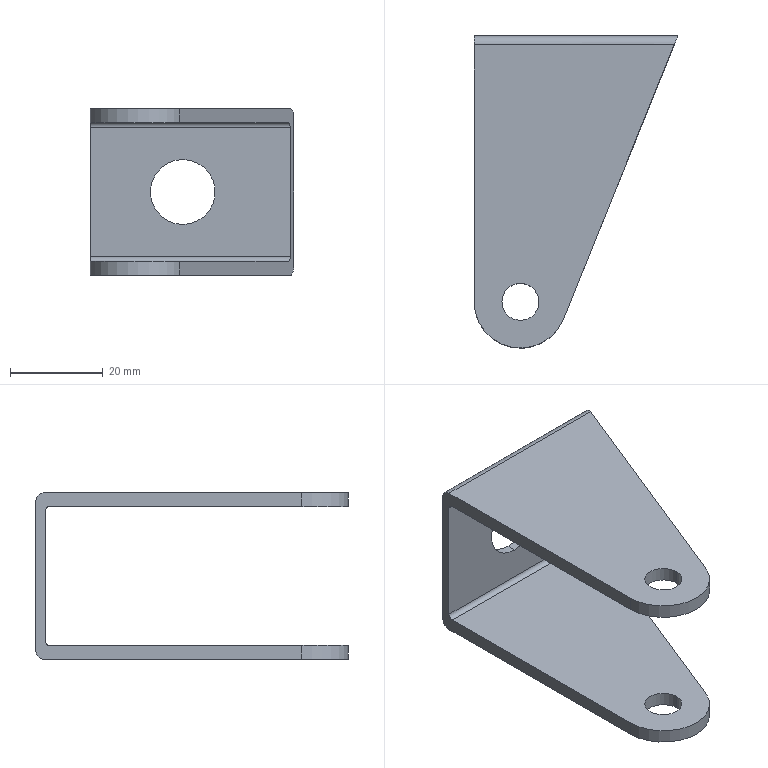Part | SolidWorks | features ICE 2, Extrusion 1, Fillet 1 | 1 solid | 20 faces | box 44 x 67.458 x 36 mm | volume 14065 mm3 | cylinder 12 | plane 8 | commonest cylinder face diameters 8 x4 2 x2 4 x2 14 x2 20 x2
STEP:
#1=CARTESIAN_POINT('',(20.,-2.,-25.));
#2=VERTEX_POINT('',#1);
#3=CARTESIAN_POINT('',(20.,-2.,-11.));
#4=VERTEX_POINT('',#3);
#5=CARTESIAN_POINT('',(20.,-2.,-18.));
#6=DIRECTION('',(0.,1.,0.));
#7=DIRECTION('',(-1.,0.,0.));
#8=AXIS2_PLACEMENT_3D('',#5,#6,#7);
#9=CIRCLE('',#8,7.);
#10=EDGE_CURVE('',#2,#4,#9,.T.);
#11=ORIENTED_EDGE('',*,*,#10,.F.);
#12=CARTESIAN_POINT('',(20.,0.,-25.));
#13=VERTEX_POINT('',#12);
#14=CARTESIAN_POINT('',(20.,-57.,-25.));
#15=DIRECTION('',(0.,1.,0.));
#16=VECTOR('',#15,1000.);
#17=LINE('',#14,#16);
#18=EDGE_CURVE('',#2,#13,#17,.T.);
#19=ORIENTED_EDGE('',*,*,#18,.T.);
#20=CARTESIAN_POINT('',(20.,0.,-11.));
#21=VERTEX_POINT('',#20);
#22=CARTESIAN_POINT('',(20.,0.,-18.));
#23=DIRECTION('',(0.,1.,0.));
#24=DIRECTION('',(0.,0.,1.));
#25=AXIS2_PLACEMENT_3D('',#22,#23,#24);
#26=CIRCLE('',#25,7.);
#27=EDGE_CURVE('',#13,#21,#26,.T.);
#28=ORIENTED_EDGE('',*,*,#27,.T.);
#29=CARTESIAN_POINT('',(20.,-57.,-11.));
#30=DIRECTION('',(0.,1.,0.));
#31=VECTOR('',#30,1000.);
#32=LINE('',#29,#31);
#33=EDGE_CURVE('',#4,#21,#32,.T.);
#34=ORIENTED_EDGE('',*,*,#33,.F.);
#35=EDGE_LOOP('',(#11,#19,#28,#34));
#36=FACE_OUTER_BOUND('',#35,.T.);
#37=CARTESIAN_POINT('',(20.,-57.,-18.));
#38=DIRECTION('',(0.,1.,0.));
#39=DIRECTION('',(0.,0.,1.));
#40=AXIS2_PLACEMENT_3D('',#37,#38,#39);
#41=CYLINDRICAL_SURFACE('',#40,7.);
#42=ADVANCED_FACE('',(#36),#41,.F.);
#43=CARTESIAN_POINT('',(14.,-57.458,-3.));
#44=VERTEX_POINT('',#43);
#45=CARTESIAN_POINT('',(6.,-57.458,-3.));
#46=VERTEX_POINT('',#45);
#47=CARTESIAN_POINT('',(10.,-57.458,-3.));
#48=DIRECTION('',(0.,0.,-1.));
#49=DIRECTION('',(0.,-1.,0.));
#50=AXIS2_PLACEMENT_3D('',#47,#48,#49);
#51=CIRCLE('',#50,4.);
#52=EDGE_CURVE('',#44,#46,#51,.T.);
#53=ORIENTED_EDGE('',*,*,#52,.T.);
#54=CARTESIAN_POINT('',(6.,-57.458,0.));
#55=VERTEX_POINT('',#54);
#56=CARTESIAN_POINT('',(6.,-57.458,-36.));
#57=DIRECTION('',(0.,0.,1.));
#58=VECTOR('',#57,1000.);
#59=LINE('',#56,#58);
#60=EDGE_CURVE('',#46,#55,#59,.T.);
#61=ORIENTED_EDGE('',*,*,#60,.T.);
#62=CARTESIAN_POINT('',(14.,-57.458,0.));
#63=VERTEX_POINT('',#62);
#64=CARTESIAN_POINT('',(10.,-57.458,0.));
#65=DIRECTION('',(0.,0.,1.));
#66=DIRECTION('',(1.,0.,0.));
#67=AXIS2_PLACEMENT_3D('',#64,#65,#66);
#68=CIRCLE('',#67,4.);
#69=EDGE_CURVE('',#55,#63,#68,.T.);
#70=ORIENTED_EDGE('',*,*,#69,.T.);
#71=CARTESIAN_POINT('',(14.,-57.458,-36.));
#72=DIRECTION('',(0.,0.,1.));
#73=VECTOR('',#72,1000.);
#74=LINE('',#71,#73);
#75=EDGE_CURVE('',#44,#63,#74,.T.);
#76=ORIENTED_EDGE('',*,*,#75,.F.);
#77=EDGE_LOOP('',(#53,#61,#70,#76));
#78=FACE_OUTER_BOUND('',#77,.T.);
#79=CARTESIAN_POINT('',(10.,-57.458,-36.));
#80=DIRECTION('',(0.,0.,1.));
#81=DIRECTION('',(1.,0.,0.));
#82=AXIS2_PLACEMENT_3D('',#79,#80,#81);
#83=CYLINDRICAL_SURFACE('',#82,4.);
#84=ADVANCED_FACE('',(#78),#83,.F.);
#85=CARTESIAN_POINT('',(6.,-57.458,-36.));
#86=VERTEX_POINT('',#85);
#87=CARTESIAN_POINT('',(14.,-57.458,-36.));
#88=VERTEX_POINT('',#87);
#89=CARTESIAN_POINT('',(10.,-57.458,-36.));
#90=DIRECTION('',(0.,0.,1.));
#91=DIRECTION('',(1.,0.,0.));
#92=AXIS2_PLACEMENT_3D('',#89,#90,#91);
#93=CIRCLE('',#92,4.);
#94=EDGE_CURVE('',#86,#88,#93,.T.);
#95=ORIENTED_EDGE('',*,*,#94,.F.);
#96=CARTESIAN_POINT('',(6.,-57.458,-33.));
#97=VERTEX_POINT('',#96);
#98=CARTESIAN_POINT('',(6.,-57.458,-36.));
#99=DIRECTION('',(0.,0.,1.));
#100=VECTOR('',#99,1000.);
#101=LINE('',#98,#100);
#102=EDGE_CURVE('',#86,#97,#101,.T.);
#103=ORIENTED_EDGE('',*,*,#102,.T.);
#104=CARTESIAN_POINT('',(14.,-57.458,-33.));
#105=VERTEX_POINT('',#104);
#106=CARTESIAN_POINT('',(10.,-57.458,-33.));
#107=DIRECTION('',(0.,0.,1.));
#108=DIRECTION('',(-1.,0.,0.));
#109=AXIS2_PLACEMENT_3D('',#106,#107,#108);
#110=CIRCLE('',#109,4.);
#111=EDGE_CURVE('',#97,#105,#110,.T.);
#112=ORIENTED_EDGE('',*,*,#111,.T.);
#113=CARTESIAN_POINT('',(14.,-57.458,-36.));
#114=DIRECTION('',(0.,0.,1.));
#115=VECTOR('',#114,1000.);
#116=LINE('',#113,#115);
#117=EDGE_CURVE('',#88,#105,#116,.T.);
#118=ORIENTED_EDGE('',*,*,#117,.F.);
#119=EDGE_LOOP('',(#95,#103,#112,#118));
#120=FACE_OUTER_BOUND('',#119,.T.);
#121=CARTESIAN_POINT('',(10.,-57.458,-36.));
#122=DIRECTION('',(0.,0.,1.));
#123=DIRECTION('',(1.,0.,0.));
#124=AXIS2_PLACEMENT_3D('',#121,#122,#123);
#125=CYLINDRICAL_SURFACE('',#124,4.);
#126=ADVANCED_FACE('',(#120),#125,.F.);
#127=CARTESIAN_POINT('',(0.,-57.458,-33.));
#128=VERTEX_POINT('',#127);
#129=CARTESIAN_POINT('',(19.272,-61.204,-33.));
#130=VERTEX_POINT('',#129);
#131=CARTESIAN_POINT('',(10.,-57.458,-33.));
#132=DIRECTION('',(0.,0.,1.));
#133=DIRECTION('',(-1.,0.,0.));
#134=AXIS2_PLACEMENT_3D('',#131,#132,#133);
#135=CIRCLE('',#134,10.);
#136=EDGE_CURVE('',#128,#130,#135,.T.);
#137=ORIENTED_EDGE('',*,*,#136,.F.);
#138=CARTESIAN_POINT('',(0.,-57.458,-36.));
#139=VERTEX_POINT('',#138);
#140=CARTESIAN_POINT('',(0.,-57.458,-36.));
#141=DIRECTION('',(0.,0.,1.));
#142=VECTOR('',#141,1000.);
#143=LINE('',#140,#142);
#144=EDGE_CURVE('',#139,#128,#143,.T.);
#145=ORIENTED_EDGE('',*,*,#144,.F.);
#146=CARTESIAN_POINT('',(19.272,-61.204,-36.));
#147=VERTEX_POINT('',#146);
#148=CARTESIAN_POINT('',(10.,-57.458,-36.));
#149=DIRECTION('',(0.,0.,1.));
#150=DIRECTION('',(1.,0.,0.));
#151=AXIS2_PLACEMENT_3D('',#148,#149,#150);
#152=CIRCLE('',#151,10.);
#153=EDGE_CURVE('',#139,#147,#152,.T.);
#154=ORIENTED_EDGE('',*,*,#153,.T.);
#155=CARTESIAN_POINT('',(19.272,-61.204,-36.));
#156=DIRECTION('',(0.,0.,1.));
#157=VECTOR('',#156,1000.);
#158=LINE('',#155,#157);
#159=EDGE_CURVE('',#147,#130,#158,.T.);
#160=ORIENTED_EDGE('',*,*,#159,.T.);
#161=EDGE_LOOP('',(#137,#145,#154,#160));
#162=FACE_OUTER_BOUND('',#161,.T.);
#163=CARTESIAN_POINT('',(10.,-57.458,-36.));
#164=DIRECTION('',(0.,0.,1.));
#165=DIRECTION('',(1.,0.,0.));
#166=AXIS2_PLACEMENT_3D('',#163,#164,#165);
#167=CYLINDRICAL_SURFACE('',#166,10.);
#168=ADVANCED_FACE('',(#162),#167,.T.);
#169=ORIENTED_EDGE('',*,*,#102,.F.);
#170=CARTESIAN_POINT('',(10.,-57.458,-36.));
#171=DIRECTION('',(0.,0.,1.));
#172=DIRECTION('',(1.,0.,0.));
#173=AXIS2_PLACEMENT_3D('',#170,#171,#172);
#174=CIRCLE('',#173,4.);
#175=EDGE_CURVE('',#88,#86,#174,.T.);
#176=ORIENTED_EDGE('',*,*,#175,.F.);
#177=ORIENTED_EDGE('',*,*,#117,.T.);
#178=CARTESIAN_POINT('',(10.,-57.458,-33.));
#179=DIRECTION('',(0.,0.,1.));
#180=DIRECTION('',(-1.,0.,0.));
#181=AXIS2_PLACEMENT_3D('',#178,#179,#180);
#182=CIRCLE('',#181,4.);
#183=EDGE_CURVE('',#105,#97,#182,.T.);
#184=ORIENTED_EDGE('',*,*,#183,.T.);
#185=EDGE_LOOP('',(#169,#176,#177,#184));
#186=FACE_OUTER_BOUND('',#185,.T.);
#187=CARTESIAN_POINT('',(10.,-57.458,-36.));
#188=DIRECTION('',(0.,0.,1.));
#189=DIRECTION('',(1.,0.,0.));
#190=AXIS2_PLACEMENT_3D('',#187,#188,#189);
#191=CYLINDRICAL_SURFACE('',#190,4.);
#192=ADVANCED_FACE('',(#186),#191,.F.);
#193=CARTESIAN_POINT('',(20.,0.,-18.));
#194=DIRECTION('',(0.,1.,0.));
#195=DIRECTION('',(0.,0.,1.));
#196=AXIS2_PLACEMENT_3D('',#193,#194,#195);
#197=CIRCLE('',#196,7.);
#198=EDGE_CURVE('',#21,#13,#197,.T.);
#199=ORIENTED_EDGE('',*,*,#198,.F.);
#200=ORIENTED_EDGE('',*,*,#27,.F.);
#201=EDGE_LOOP('',(#199,#200));
#202=FACE_BOUND('',#201,.T.);
#203=CARTESIAN_POINT('',(0.,0.,-34.));
#204=VERTEX_POINT('',#203);
#205=CARTESIAN_POINT('',(0.,0.,-2.));
#206=VERTEX_POINT('',#205);
#207=CARTESIAN_POINT('',(0.,0.,-36.));
#208=DIRECTION('',(0.,0.,1.));
#209=VECTOR('',#208,1000.);
#210=LINE('',#207,#209);
#211=EDGE_CURVE('',#204,#206,#210,.T.);
#212=ORIENTED_EDGE('',*,*,#211,.T.);
#213=CARTESIAN_POINT('',(44.,0.,-2.));
#214=VERTEX_POINT('',#213);
#215=CARTESIAN_POINT('',(0.,0.,-2.));
#216=DIRECTION('',(1.,0.,0.));
#217=VECTOR('',#216,1000.);
#218=LINE('',#215,#217);
#219=EDGE_CURVE('',#206,#214,#218,.T.);
#220=ORIENTED_EDGE('',*,*,#219,.T.);
#221=CARTESIAN_POINT('',(44.,0.,-34.));
#222=VERTEX_POINT('',#221);
#223=CARTESIAN_POINT('',(44.,0.,-36.));
#224=DIRECTION('',(0.,0.,1.));
#225=VECTOR('',#224,1000.);
#226=LINE('',#223,#225);
#227=EDGE_CURVE('',#222,#214,#226,.T.);
#228=ORIENTED_EDGE('',*,*,#227,.F.);
#229=CARTESIAN_POINT('',(0.,0.,-34.));
#230=DIRECTION('',(-1.,0.,0.));
#231=VECTOR('',#230,1000.);
#232=LINE('',#229,#231);
#233=EDGE_CURVE('',#222,#204,#232,.T.);
#234=ORIENTED_EDGE('',*,*,#233,.T.);
#235=EDGE_LOOP('',(#212,#220,#228,#234));
#236=FACE_OUTER_BOUND('',#235,.T.);
#237=CARTESIAN_POINT('',(0.,0.,-36.));
#238=DIRECTION('',(0.,1.,0.));
#239=DIRECTION('',(0.,0.,1.));
#240=AXIS2_PLACEMENT_3D('',#237,#238,#239);
#241=PLANE('',#240);
#242=ADVANCED_FACE('',(#202,#236),#241,.T.);
#243=ORIENTED_EDGE('',*,*,#227,.T.);
#244=CARTESIAN_POINT('',(43.192,-2.,0.));
#245=VERTEX_POINT('',#244);
#246=CARTESIAN_POINT('',(44.,0.,-2.));
#247=CARTESIAN_POINT('',(44.,0.,-0.8284));
#248=CARTESIAN_POINT('',(43.665,-0.8284,0.));
#249=CARTESIAN_POINT('',(43.192,-2.,0.));
#250=(BOUNDED_CURVE()B_SPLINE_CURVE(3,(#246,#247,#248,#249),.UNSPECIFIED.,.F.,.F.)B_SPLINE_CURVE_WITH_KNOTS((4,4),(3.142,4.712),.UNSPECIFIED.)CURVE()GEOMETRIC_REPRESENTATION_ITEM()RATIONAL_B_SPLINE_CURVE((1.,0.8047,0.8047,1.))REPRESENTATION_ITEM(''));
#251=EDGE_CURVE('',#214,#245,#250,.T.);
#252=ORIENTED_EDGE('',*,*,#251,.T.);
#253=CARTESIAN_POINT('',(19.272,-61.204,0.));
#254=VERTEX_POINT('',#253);
#255=CARTESIAN_POINT('',(44.,0.,0.));
#256=DIRECTION('',(0.3746,0.9272,0.));
#257=VECTOR('',#256,1000.);
#258=LINE('',#255,#257);
#259=EDGE_CURVE('',#254,#245,#258,.T.);
#260=ORIENTED_EDGE('',*,*,#259,.F.);
#261=CARTESIAN_POINT('',(19.272,-61.204,-3.));
#262=VERTEX_POINT('',#261);
#263=CARTESIAN_POINT('',(19.272,-61.204,-36.));
#264=DIRECTION('',(0.,0.,1.));
#265=VECTOR('',#264,1000.);
#266=LINE('',#263,#265);
#267=EDGE_CURVE('',#262,#254,#266,.T.);
#268=ORIENTED_EDGE('',*,*,#267,.F.);
#269=CARTESIAN_POINT('',(42.788,-3.,-3.));
#270=VERTEX_POINT('',#269);
#271=CARTESIAN_POINT('',(44.,0.,-3.));
#272=DIRECTION('',(-0.3746,-0.9272,0.));
#273=VECTOR('',#272,1000.);
#274=LINE('',#271,#273);
#275=EDGE_CURVE('',#270,#262,#274,.T.);
#276=ORIENTED_EDGE('',*,*,#275,.F.);
#277=CARTESIAN_POINT('',(43.192,-2.,-4.));
#278=VERTEX_POINT('',#277);
#279=CARTESIAN_POINT('',(43.192,-2.,-4.));
#280=CARTESIAN_POINT('',(43.192,-2.,-3.414));
#281=CARTESIAN_POINT('',(43.025,-2.414,-3.));
#282=CARTESIAN_POINT('',(42.788,-3.,-3.));
#283=(BOUNDED_CURVE()B_SPLINE_CURVE(3,(#279,#280,#281,#282),.UNSPECIFIED.,.F.,.F.)B_SPLINE_CURVE_WITH_KNOTS((4,4),(3.142,4.712),.UNSPECIFIED.)CURVE()GEOMETRIC_REPRESENTATION_ITEM()RATIONAL_B_SPLINE_CURVE((1.,0.8047,0.8047,1.))REPRESENTATION_ITEM(''));
#284=EDGE_CURVE('',#278,#270,#283,.T.);
#285=ORIENTED_EDGE('',*,*,#284,.F.);
#286=CARTESIAN_POINT('',(43.192,-2.,-32.));
#287=VERTEX_POINT('',#286);
#288=CARTESIAN_POINT('',(43.192,-2.,-36.));
#289=DIRECTION('',(0.,0.,1.));
#290=VECTOR('',#289,1000.);
#291=LINE('',#288,#290);
#292=EDGE_CURVE('',#287,#278,#291,.T.);
#293=ORIENTED_EDGE('',*,*,#292,.F.);
#294=CARTESIAN_POINT('',(42.788,-3.,-33.));
#295=VERTEX_POINT('',#294);
#296=CARTESIAN_POINT('',(42.788,-3.,-33.));
#297=CARTESIAN_POINT('',(43.025,-2.414,-33.));
#298=CARTESIAN_POINT('',(43.192,-2.,-32.586));
#299=CARTESIAN_POINT('',(43.192,-2.,-32.));
#300=(BOUNDED_CURVE()B_SPLINE_CURVE(3,(#296,#297,#298,#299),.UNSPECIFIED.,.F.,.F.)B_SPLINE_CURVE_WITH_KNOTS((4,4),(1.571,3.142),.UNSPECIFIED.)CURVE()GEOMETRIC_REPRESENTATION_ITEM()RATIONAL_B_SPLINE_CURVE((1.,0.8047,0.8047,1.))REPRESENTATION_ITEM(''));
#301=EDGE_CURVE('',#295,#287,#300,.T.);
#302=ORIENTED_EDGE('',*,*,#301,.F.);
#303=CARTESIAN_POINT('',(44.,0.,-33.));
#304=DIRECTION('',(0.3746,0.9272,0.));
#305=VECTOR('',#304,1000.);
#306=LINE('',#303,#305);
#307=EDGE_CURVE('',#130,#295,#306,.T.);
#308=ORIENTED_EDGE('',*,*,#307,.F.);
#309=ORIENTED_EDGE('',*,*,#159,.F.);
#310=CARTESIAN_POINT('',(43.192,-2.,-36.));
#311=VERTEX_POINT('',#310);
#312=CARTESIAN_POINT('',(44.,0.,-36.));
#313=DIRECTION('',(0.3746,0.9272,0.));
#314=VECTOR('',#313,1000.);
#315=LINE('',#312,#314);
#316=EDGE_CURVE('',#147,#311,#315,.T.);
#317=ORIENTED_EDGE('',*,*,#316,.T.);
#318=CARTESIAN_POINT('',(43.192,-2.,-36.));
#319=CARTESIAN_POINT('',(43.665,-0.8284,-36.));
#320=CARTESIAN_POINT('',(44.,0.,-35.172));
#321=CARTESIAN_POINT('',(44.,0.,-34.));
#322=(BOUNDED_CURVE()B_SPLINE_CURVE(3,(#318,#319,#320,#321),.UNSPECIFIED.,.F.,.F.)B_SPLINE_CURVE_WITH_KNOTS((4,4),(4.712,6.283),.UNSPECIFIED.)CURVE()GEOMETRIC_REPRESENTATION_ITEM()RATIONAL_B_SPLINE_CURVE((1.,0.8047,0.8047,1.))REPRESENTATION_ITEM(''));
#323=EDGE_CURVE('',#311,#222,#322,.T.);
#324=ORIENTED_EDGE('',*,*,#323,.T.);
#325=EDGE_LOOP('',(#243,#252,#260,#268,#276,#285,#293,#302,#308,#309,#317,#324));
#326=FACE_OUTER_BOUND('',#325,.T.);
#327=CARTESIAN_POINT('',(44.,0.,-36.));
#328=DIRECTION('',(0.9272,-0.3746,0.));
#329=DIRECTION('',(0.3746,0.9272,0.));
#330=AXIS2_PLACEMENT_3D('',#327,#328,#329);
#331=PLANE('',#330);
#332=ADVANCED_FACE('',(#326),#331,.T.);
#333=CARTESIAN_POINT('',(0.,-57.458,-3.));
#334=VERTEX_POINT('',#333);
#335=CARTESIAN_POINT('',(10.,-57.458,-3.));
#336=DIRECTION('',(0.,0.,-1.));
#337=DIRECTION('',(0.,-1.,0.));
#338=AXIS2_PLACEMENT_3D('',#335,#336,#337);
#339=CIRCLE('',#338,10.);
#340=EDGE_CURVE('',#262,#334,#339,.T.);
#341=ORIENTED_EDGE('',*,*,#340,.F.);
#342=ORIENTED_EDGE('',*,*,#267,.T.);
#343=CARTESIAN_POINT('',(0.,-57.458,0.));
#344=VERTEX_POINT('',#343);
#345=CARTESIAN_POINT('',(10.,-57.458,0.));
#346=DIRECTION('',(0.,0.,1.));
#347=DIRECTION('',(1.,0.,0.));
#348=AXIS2_PLACEMENT_3D('',#345,#346,#347);
#349=CIRCLE('',#348,10.);
#350=EDGE_CURVE('',#344,#254,#349,.T.);
#351=ORIENTED_EDGE('',*,*,#350,.F.);
#352=CARTESIAN_POINT('',(0.,-57.458,-36.));
#353=DIRECTION('',(0.,0.,1.));
#354=VECTOR('',#353,1000.);
#355=LINE('',#352,#354);
#356=EDGE_CURVE('',#334,#344,#355,.T.);
#357=ORIENTED_EDGE('',*,*,#356,.F.);
#358=EDGE_LOOP('',(#341,#342,#351,#357));
#359=FACE_OUTER_BOUND('',#358,.T.);
#360=CARTESIAN_POINT('',(10.,-57.458,-36.));
#361=DIRECTION('',(0.,0.,1.));
#362=DIRECTION('',(1.,0.,0.));
#363=AXIS2_PLACEMENT_3D('',#360,#361,#362);
#364=CYLINDRICAL_SURFACE('',#363,10.);
#365=ADVANCED_FACE('',(#359),#364,.T.);
#366=CARTESIAN_POINT('',(0.,-2.,0.));
#367=VERTEX_POINT('',#366);
#368=CARTESIAN_POINT('',(0.,0.,0.));
#369=DIRECTION('',(0.,-1.,0.));
#370=VECTOR('',#369,1000.);
#371=LINE('',#368,#370);
#372=EDGE_CURVE('',#367,#344,#371,.T.);
#373=ORIENTED_EDGE('',*,*,#372,.F.);
#374=CARTESIAN_POINT('',(0.,-2.,-2.));
#375=DIRECTION('',(-1.,0.,0.));
#376=DIRECTION('',(0.,-1.,0.));
#377=AXIS2_PLACEMENT_3D('',#374,#375,#376);
#378=CIRCLE('',#377,2.);
#379=EDGE_CURVE('',#367,#206,#378,.T.);
#380=ORIENTED_EDGE('',*,*,#379,.T.);
#381=ORIENTED_EDGE('',*,*,#211,.F.);
#382=CARTESIAN_POINT('',(0.,-2.,-36.));
#383=VERTEX_POINT('',#382);
#384=CARTESIAN_POINT('',(0.,-2.,-34.));
#385=DIRECTION('',(-1.,0.,0.));
#386=DIRECTION('',(0.,-1.,0.));
#387=AXIS2_PLACEMENT_3D('',#384,#385,#386);
#388=CIRCLE('',#387,2.);
#389=EDGE_CURVE('',#204,#383,#388,.T.);
#390=ORIENTED_EDGE('',*,*,#389,.T.);
#391=CARTESIAN_POINT('',(0.,0.,-36.));
#392=DIRECTION('',(0.,-1.,0.));
#393=VECTOR('',#392,1000.);
#394=LINE('',#391,#393);
#395=EDGE_CURVE('',#383,#139,#394,.T.);
#396=ORIENTED_EDGE('',*,*,#395,.T.);
#397=ORIENTED_EDGE('',*,*,#144,.T.);
#398=CARTESIAN_POINT('',(0.,-3.,-33.));
#399=VERTEX_POINT('',#398);
#400=CARTESIAN_POINT('',(0.,-3.,-33.));
#401=DIRECTION('',(0.,-1.,0.));
#402=VECTOR('',#401,1000.);
#403=LINE('',#400,#402);
#404=EDGE_CURVE('',#399,#128,#403,.T.);
#405=ORIENTED_EDGE('',*,*,#404,.F.);
#406=CARTESIAN_POINT('',(0.,-2.,-32.));
#407=VERTEX_POINT('',#406);
#408=CARTESIAN_POINT('',(0.,-3.,-32.));
#409=DIRECTION('',(-1.,0.,0.));
#410=DIRECTION('',(0.,1.,0.));
#411=AXIS2_PLACEMENT_3D('',#408,#409,#410);
#412=CIRCLE('',#411,1.);
#413=EDGE_CURVE('',#407,#399,#412,.T.);
#414=ORIENTED_EDGE('',*,*,#413,.F.);
#415=CARTESIAN_POINT('',(0.,-2.,-4.));
#416=VERTEX_POINT('',#415);
#417=CARTESIAN_POINT('',(0.,-2.,-32.));
#418=DIRECTION('',(0.,0.,-1.));
#419=VECTOR('',#418,1000.);
#420=LINE('',#417,#419);
#421=EDGE_CURVE('',#416,#407,#420,.T.);
#422=ORIENTED_EDGE('',*,*,#421,.F.);
#423=CARTESIAN_POINT('',(0.,-3.,-3.));
#424=VERTEX_POINT('',#423);
#425=CARTESIAN_POINT('',(0.,-3.,-4.));
#426=DIRECTION('',(-1.,0.,0.));
#427=DIRECTION('',(0.,-1.,0.));
#428=AXIS2_PLACEMENT_3D('',#425,#426,#427);
#429=CIRCLE('',#428,1.);
#430=EDGE_CURVE('',#424,#416,#429,.T.);
#431=ORIENTED_EDGE('',*,*,#430,.F.);
#432=CARTESIAN_POINT('',(0.,-3.,-3.));
#433=DIRECTION('',(0.,1.,0.));
#434=VECTOR('',#433,1000.);
#435=LINE('',#432,#434);
#436=EDGE_CURVE('',#334,#424,#435,.T.);
#437=ORIENTED_EDGE('',*,*,#436,.F.);
#438=ORIENTED_EDGE('',*,*,#356,.T.);
#439=EDGE_LOOP('',(#373,#380,#381,#390,#396,#397,#405,#414,#422,#431,#437,#438));
#440=FACE_OUTER_BOUND('',#439,.T.);
#441=CARTESIAN_POINT('',(0.,0.,-36.));
#442=DIRECTION('',(-1.,0.,0.));
#443=DIRECTION('',(0.,-1.,0.));
#444=AXIS2_PLACEMENT_3D('',#441,#442,#443);
#445=PLANE('',#444);
#446=ADVANCED_FACE('',(#440),#445,.T.);
#447=ORIENTED_EDGE('',*,*,#175,.T.);
#448=ORIENTED_EDGE('',*,*,#94,.T.);
#449=EDGE_LOOP('',(#447,#448));
#450=FACE_BOUND('',#449,.T.);
#451=ORIENTED_EDGE('',*,*,#395,.F.);
#452=CARTESIAN_POINT('',(44.,-2.,-36.));
#453=DIRECTION('',(1.,0.,0.));
#454=VECTOR('',#453,1000.);
#455=LINE('',#452,#454);
#456=EDGE_CURVE('',#383,#311,#455,.T.);
#457=ORIENTED_EDGE('',*,*,#456,.T.);
#458=ORIENTED_EDGE('',*,*,#316,.F.);
#459=ORIENTED_EDGE('',*,*,#153,.F.);
#460=EDGE_LOOP('',(#451,#457,#458,#459));
#461=FACE_OUTER_BOUND('',#460,.T.);
#462=CARTESIAN_POINT('',(10.,-57.458,-36.));
#463=DIRECTION('',(0.,0.,1.));
#464=DIRECTION('',(1.,0.,0.));
#465=AXIS2_PLACEMENT_3D('',#462,#463,#464);
#466=PLANE('',#465);
#467=ADVANCED_FACE('',(#450,#461),#466,.F.);
#468=CARTESIAN_POINT('',(10.,-57.458,0.));
#469=DIRECTION('',(0.,0.,1.));
#470=DIRECTION('',(1.,0.,0.));
#471=AXIS2_PLACEMENT_3D('',#468,#469,#470);
#472=CIRCLE('',#471,4.);
#473=EDGE_CURVE('',#63,#55,#472,.T.);
#474=ORIENTED_EDGE('',*,*,#473,.F.);
#475=ORIENTED_EDGE('',*,*,#69,.F.);
#476=EDGE_LOOP('',(#474,#475));
#477=FACE_BOUND('',#476,.T.);
#478=ORIENTED_EDGE('',*,*,#259,.T.);
#479=CARTESIAN_POINT('',(10.,-2.,0.));
#480=DIRECTION('',(-1.,0.,0.));
#481=VECTOR('',#480,1000.);
#482=LINE('',#479,#481);
#483=EDGE_CURVE('',#245,#367,#482,.T.);
#484=ORIENTED_EDGE('',*,*,#483,.T.);
#485=ORIENTED_EDGE('',*,*,#372,.T.);
#486=ORIENTED_EDGE('',*,*,#350,.T.);
#487=EDGE_LOOP('',(#478,#484,#485,#486));
#488=FACE_OUTER_BOUND('',#487,.T.);
#489=CARTESIAN_POINT('',(10.,-57.458,0.));
#490=DIRECTION('',(0.,0.,1.));
#491=DIRECTION('',(1.,0.,0.));
#492=AXIS2_PLACEMENT_3D('',#489,#490,#491);
#493=PLANE('',#492);
#494=ADVANCED_FACE('',(#477,#488),#493,.T.);
#495=ORIENTED_EDGE('',*,*,#60,.F.);
#496=CARTESIAN_POINT('',(10.,-57.458,-3.));
#497=DIRECTION('',(0.,0.,-1.));
#498=DIRECTION('',(0.,-1.,0.));
#499=AXIS2_PLACEMENT_3D('',#496,#497,#498);
#500=CIRCLE('',#499,4.);
#501=EDGE_CURVE('',#46,#44,#500,.T.);
#502=ORIENTED_EDGE('',*,*,#501,.T.);
#503=ORIENTED_EDGE('',*,*,#75,.T.);
#504=ORIENTED_EDGE('',*,*,#473,.T.);
#505=EDGE_LOOP('',(#495,#502,#503,#504));
#506=FACE_OUTER_BOUND('',#505,.T.);
#507=CARTESIAN_POINT('',(10.,-57.458,-36.));
#508=DIRECTION('',(0.,0.,1.));
#509=DIRECTION('',(1.,0.,0.));
#510=AXIS2_PLACEMENT_3D('',#507,#508,#509);
#511=CYLINDRICAL_SURFACE('',#510,4.);
#512=ADVANCED_FACE('',(#506),#511,.F.);
#513=ORIENTED_EDGE('',*,*,#307,.T.);
#514=CARTESIAN_POINT('',(57.,-3.,-33.));
#515=DIRECTION('',(-1.,0.,0.));
#516=VECTOR('',#515,1000.);
#517=LINE('',#514,#516);
#518=EDGE_CURVE('',#295,#399,#517,.T.);
#519=ORIENTED_EDGE('',*,*,#518,.T.);
#520=ORIENTED_EDGE('',*,*,#404,.T.);
#521=ORIENTED_EDGE('',*,*,#136,.T.);
#522=EDGE_LOOP('',(#513,#519,#520,#521));
#523=FACE_OUTER_BOUND('',#522,.T.);
#524=ORIENTED_EDGE('',*,*,#183,.F.);
#525=ORIENTED_EDGE('',*,*,#111,.F.);
#526=EDGE_LOOP('',(#524,#525));
#527=FACE_BOUND('',#526,.T.);
#528=CARTESIAN_POINT('',(57.,-3.,-33.));
#529=DIRECTION('',(0.,0.,-1.));
#530=DIRECTION('',(-1.,0.,0.));
#531=AXIS2_PLACEMENT_3D('',#528,#529,#530);
#532=PLANE('',#531);
#533=ADVANCED_FACE('',(#523,#527),#532,.F.);
#534=ORIENTED_EDGE('',*,*,#275,.T.);
#535=ORIENTED_EDGE('',*,*,#340,.T.);
#536=ORIENTED_EDGE('',*,*,#436,.T.);
#537=CARTESIAN_POINT('',(57.,-3.,-3.));
#538=DIRECTION('',(-1.,0.,0.));
#539=VECTOR('',#538,1000.);
#540=LINE('',#537,#539);
#541=EDGE_CURVE('',#270,#424,#540,.T.);
#542=ORIENTED_EDGE('',*,*,#541,.F.);
#543=EDGE_LOOP('',(#534,#535,#536,#542));
#544=FACE_OUTER_BOUND('',#543,.T.);
#545=ORIENTED_EDGE('',*,*,#52,.F.);
#546=ORIENTED_EDGE('',*,*,#501,.F.);
#547=EDGE_LOOP('',(#545,#546));
#548=FACE_BOUND('',#547,.T.);
#549=CARTESIAN_POINT('',(57.,-3.,-3.));
#550=DIRECTION('',(0.,0.,1.));
#551=DIRECTION('',(0.,-1.,0.));
#552=AXIS2_PLACEMENT_3D('',#549,#550,#551);
#553=PLANE('',#552);
#554=ADVANCED_FACE('',(#544,#548),#553,.F.);
#555=ORIENTED_EDGE('',*,*,#301,.T.);
#556=CARTESIAN_POINT('',(57.,-2.,-32.));
#557=DIRECTION('',(-1.,0.,0.));
#558=VECTOR('',#557,1000.);
#559=LINE('',#556,#558);
#560=EDGE_CURVE('',#287,#407,#559,.T.);
#561=ORIENTED_EDGE('',*,*,#560,.T.);
#562=ORIENTED_EDGE('',*,*,#413,.T.);
#563=ORIENTED_EDGE('',*,*,#518,.F.);
#564=EDGE_LOOP('',(#555,#561,#562,#563));
#565=FACE_OUTER_BOUND('',#564,.T.);
#566=CARTESIAN_POINT('',(57.,-3.,-32.));
#567=DIRECTION('',(-1.,0.,0.));
#568=DIRECTION('',(0.,-1.,0.));
#569=AXIS2_PLACEMENT_3D('',#566,#567,#568);
#570=CYLINDRICAL_SURFACE('',#569,1.);
#571=ADVANCED_FACE('',(#565),#570,.F.);
#572=CARTESIAN_POINT('',(20.,-2.,-18.));
#573=DIRECTION('',(0.,1.,0.));
#574=DIRECTION('',(-1.,0.,0.));
#575=AXIS2_PLACEMENT_3D('',#572,#573,#574);
#576=CIRCLE('',#575,7.);
#577=EDGE_CURVE('',#4,#2,#576,.T.);
#578=ORIENTED_EDGE('',*,*,#577,.T.);
#579=ORIENTED_EDGE('',*,*,#10,.T.);
#580=EDGE_LOOP('',(#578,#579));
#581=FACE_BOUND('',#580,.T.);
#582=ORIENTED_EDGE('',*,*,#292,.T.);
#583=CARTESIAN_POINT('',(57.,-2.,-4.));
#584=DIRECTION('',(-1.,0.,0.));
#585=VECTOR('',#584,1000.);
#586=LINE('',#583,#585);
#587=EDGE_CURVE('',#278,#416,#586,.T.);
#588=ORIENTED_EDGE('',*,*,#587,.T.);
#589=ORIENTED_EDGE('',*,*,#421,.T.);
#590=ORIENTED_EDGE('',*,*,#560,.F.);
#591=EDGE_LOOP('',(#582,#588,#589,#590));
#592=FACE_OUTER_BOUND('',#591,.T.);
#593=CARTESIAN_POINT('',(57.,-2.,-32.));
#594=DIRECTION('',(0.,1.,0.));
#595=DIRECTION('',(-1.,0.,0.));
#596=AXIS2_PLACEMENT_3D('',#593,#594,#595);
#597=PLANE('',#596);
#598=ADVANCED_FACE('',(#581,#592),#597,.F.);
#599=ORIENTED_EDGE('',*,*,#284,.T.);
#600=ORIENTED_EDGE('',*,*,#541,.T.);
#601=ORIENTED_EDGE('',*,*,#430,.T.);
#602=ORIENTED_EDGE('',*,*,#587,.F.);
#603=EDGE_LOOP('',(#599,#600,#601,#602));
#604=FACE_OUTER_BOUND('',#603,.T.);
#605=CARTESIAN_POINT('',(57.,-3.,-4.));
#606=DIRECTION('',(-1.,0.,0.));
#607=DIRECTION('',(0.,-1.,0.));
#608=AXIS2_PLACEMENT_3D('',#605,#606,#607);
#609=CYLINDRICAL_SURFACE('',#608,1.);
#610=ADVANCED_FACE('',(#604),#609,.F.);
#611=ORIENTED_EDGE('',*,*,#251,.F.);
#612=ORIENTED_EDGE('',*,*,#219,.F.);
#613=ORIENTED_EDGE('',*,*,#379,.F.);
#614=ORIENTED_EDGE('',*,*,#483,.F.);
#615=EDGE_LOOP('',(#611,#612,#613,#614));
#616=FACE_OUTER_BOUND('',#615,.T.);
#617=CARTESIAN_POINT('',(10.,-2.,-2.));
#618=DIRECTION('',(-1.,0.,0.));
#619=DIRECTION('',(0.,0.,1.));
#620=AXIS2_PLACEMENT_3D('',#617,#618,#619);
#621=CYLINDRICAL_SURFACE('',#620,2.);
#622=ADVANCED_FACE('',(#616),#621,.T.);
#623=ORIENTED_EDGE('',*,*,#323,.F.);
#624=ORIENTED_EDGE('',*,*,#456,.F.);
#625=ORIENTED_EDGE('',*,*,#389,.F.);
#626=ORIENTED_EDGE('',*,*,#233,.F.);
#627=EDGE_LOOP('',(#623,#624,#625,#626));
#628=FACE_OUTER_BOUND('',#627,.T.);
#629=CARTESIAN_POINT('',(0.,-2.,-34.));
#630=DIRECTION('',(1.,0.,0.));
#631=DIRECTION('',(0.,0.,-1.));
#632=AXIS2_PLACEMENT_3D('',#629,#630,#631);
#633=CYLINDRICAL_SURFACE('',#632,2.);
#634=ADVANCED_FACE('',(#628),#633,.T.);
#635=ORIENTED_EDGE('',*,*,#18,.F.);
#636=ORIENTED_EDGE('',*,*,#577,.F.);
#637=ORIENTED_EDGE('',*,*,#33,.T.);
#638=ORIENTED_EDGE('',*,*,#198,.T.);
#639=EDGE_LOOP('',(#635,#636,#637,#638));
#640=FACE_OUTER_BOUND('',#639,.T.);
#641=CARTESIAN_POINT('',(20.,-57.,-18.));
#642=DIRECTION('',(0.,1.,0.));
#643=DIRECTION('',(0.,0.,1.));
#644=AXIS2_PLACEMENT_3D('',#641,#642,#643);
#645=CYLINDRICAL_SURFACE('',#644,7.);
#646=ADVANCED_FACE('',(#640),#645,.F.);
#647=CLOSED_SHELL('',(#42,#84,#126,#168,#192,#242,#332,#365,#446,#467,#494,#512,#533,#554,#571,#598,#610,#622,#634,#646));
#648=MANIFOLD_SOLID_BREP('',#647);
#649=CARTESIAN_POINT('',(0.,0.,0.));
#650=DIRECTION('',(0.,0.,1.));
#651=DIRECTION('',(1.,0.,0.));
#652=AXIS2_PLACEMENT_3D('',#649,#650,#651);
#653=(LENGTH_UNIT()NAMED_UNIT(*)SI_UNIT(.MILLI.,.METRE.));
#654=UNCERTAINTY_MEASURE_WITH_UNIT(LENGTH_MEASURE(0.00001),#653,'','');
#655=(NAMED_UNIT(*)PLANE_ANGLE_UNIT()SI_UNIT($,.RADIAN.));
#656=(NAMED_UNIT(*)SI_UNIT($,.STERADIAN.)SOLID_ANGLE_UNIT());
#657=(GEOMETRIC_REPRESENTATION_CONTEXT(3)GLOBAL_UNCERTAINTY_ASSIGNED_CONTEXT((#654))GLOBAL_UNIT_ASSIGNED_CONTEXT((#653,#655,#656))REPRESENTATION_CONTEXT('',''));
#658=ADVANCED_BREP_SHAPE_REPRESENTATION('',(#648,#652),#657);